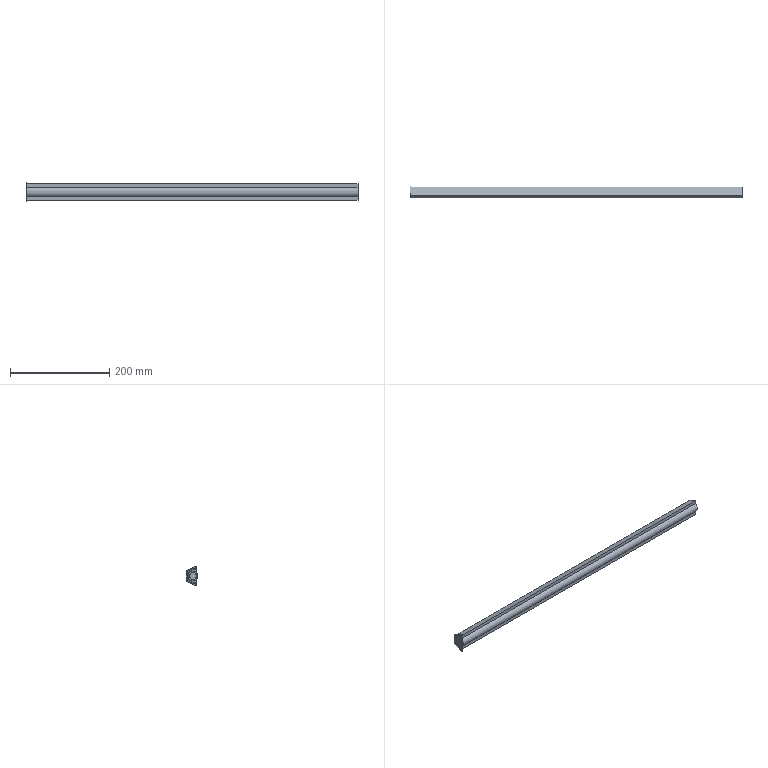Part | SolidWorks | features BaseBody 2, ICE 1 | 2 solids | 25 faces | box 670 x 24 x 40.186 mm | volume 190097 mm3 | plane 21 | cylinder 4 | commonest cylinder face diameters 14 x2 20 x2
STEP:
#1=CARTESIAN_POINT('',(-503.717,-23.698,18.335));
#2=VERTEX_POINT('',#1);
#3=CARTESIAN_POINT('',(-1171.717,-23.698,18.335));
#4=VERTEX_POINT('',#3);
#5=CARTESIAN_POINT('',(-6.717,-23.698,18.335));
#6=DIRECTION('',(-1.,0.,0.));
#7=VECTOR('',#6,1000.);
#8=LINE('',#5,#7);
#9=EDGE_CURVE('',#2,#4,#8,.T.);
#10=ORIENTED_EDGE('',*,*,#9,.F.);
#11=CARTESIAN_POINT('',(-503.717,-25.698,18.335));
#12=VERTEX_POINT('',#11);
#13=CARTESIAN_POINT('',(-503.717,-23.698,18.335));
#14=DIRECTION('',(0.,-1.,0.));
#15=VECTOR('',#14,1000.);
#16=LINE('',#13,#15);
#17=EDGE_CURVE('',#2,#12,#16,.T.);
#18=ORIENTED_EDGE('',*,*,#17,.T.);
#19=CARTESIAN_POINT('',(-1171.717,-25.698,18.335));
#20=VERTEX_POINT('',#19);
#21=CARTESIAN_POINT('',(-1171.717,-25.698,18.335));
#22=DIRECTION('',(1.,0.,0.));
#23=VECTOR('',#22,1000.);
#24=LINE('',#21,#23);
#25=EDGE_CURVE('',#20,#12,#24,.T.);
#26=ORIENTED_EDGE('',*,*,#25,.F.);
#27=CARTESIAN_POINT('',(-1171.717,-23.698,18.335));
#28=DIRECTION('',(0.,-1.,0.));
#29=VECTOR('',#28,1000.);
#30=LINE('',#27,#29);
#31=EDGE_CURVE('',#4,#20,#30,.T.);
#32=ORIENTED_EDGE('',*,*,#31,.F.);
#33=EDGE_LOOP('',(#10,#18,#26,#32));
#34=FACE_OUTER_BOUND('',#33,.T.);
#35=CARTESIAN_POINT('',(-6.717,-23.698,18.335));
#36=DIRECTION('',(0.,0.,-1.));
#37=DIRECTION('',(-1.,0.,0.));
#38=AXIS2_PLACEMENT_3D('',#35,#36,#37);
#39=PLANE('',#38);
#40=ADVANCED_FACE('',(#34),#39,.T.);
#41=CARTESIAN_POINT('',(-503.717,-8.698,17.685));
#42=VERTEX_POINT('',#41);
#43=CARTESIAN_POINT('',(-1171.717,-8.698,17.685));
#44=VERTEX_POINT('',#43);
#45=CARTESIAN_POINT('',(-6.717,-8.698,17.685));
#46=DIRECTION('',(-1.,0.,0.));
#47=VECTOR('',#46,1000.);
#48=LINE('',#45,#47);
#49=EDGE_CURVE('',#42,#44,#48,.T.);
#50=ORIENTED_EDGE('',*,*,#49,.F.);
#51=CARTESIAN_POINT('',(-503.717,-8.698,-1.015));
#52=VERTEX_POINT('',#51);
#53=CARTESIAN_POINT('',(-503.717,-8.698,17.685));
#54=DIRECTION('',(0.,0.,-1.));
#55=VECTOR('',#54,1000.);
#56=LINE('',#53,#55);
#57=EDGE_CURVE('',#42,#52,#56,.T.);
#58=ORIENTED_EDGE('',*,*,#57,.T.);
#59=CARTESIAN_POINT('',(-1171.717,-8.698,-1.015));
#60=VERTEX_POINT('',#59);
#61=CARTESIAN_POINT('',(-1171.717,-8.698,-1.015));
#62=DIRECTION('',(1.,0.,0.));
#63=VECTOR('',#62,1000.);
#64=LINE('',#61,#63);
#65=EDGE_CURVE('',#60,#52,#64,.T.);
#66=ORIENTED_EDGE('',*,*,#65,.F.);
#67=CARTESIAN_POINT('',(-1171.717,-8.698,17.685));
#68=DIRECTION('',(0.,0.,-1.));
#69=VECTOR('',#68,1000.);
#70=LINE('',#67,#69);
#71=EDGE_CURVE('',#44,#60,#70,.T.);
#72=ORIENTED_EDGE('',*,*,#71,.F.);
#73=EDGE_LOOP('',(#50,#58,#66,#72));
#74=FACE_OUTER_BOUND('',#73,.T.);
#75=CARTESIAN_POINT('',(-6.717,-8.698,17.685));
#76=DIRECTION('',(0.,1.,0.));
#77=DIRECTION('',(0.,0.,-1.));
#78=AXIS2_PLACEMENT_3D('',#75,#76,#77);
#79=PLANE('',#78);
#80=ADVANCED_FACE('',(#74),#79,.T.);
#81=ORIENTED_EDGE('',*,*,#65,.T.);
#82=CARTESIAN_POINT('',(-503.717,-25.698,-8.665));
#83=VERTEX_POINT('',#82);
#84=CARTESIAN_POINT('',(-503.717,-8.698,-1.015));
#85=DIRECTION('',(0.,-0.9119,-0.4104));
#86=VECTOR('',#85,1000.);
#87=LINE('',#84,#86);
#88=EDGE_CURVE('',#52,#83,#87,.T.);
#89=ORIENTED_EDGE('',*,*,#88,.T.);
#90=CARTESIAN_POINT('',(-1171.717,-25.698,-8.665));
#91=VERTEX_POINT('',#90);
#92=CARTESIAN_POINT('',(-1171.717,-25.698,-8.665));
#93=DIRECTION('',(1.,0.,0.));
#94=VECTOR('',#93,1000.);
#95=LINE('',#92,#94);
#96=EDGE_CURVE('',#91,#83,#95,.T.);
#97=ORIENTED_EDGE('',*,*,#96,.F.);
#98=CARTESIAN_POINT('',(-1171.717,-8.698,-1.015));
#99=DIRECTION('',(0.,-0.9119,-0.4104));
#100=VECTOR('',#99,1000.);
#101=LINE('',#98,#100);
#102=EDGE_CURVE('',#60,#91,#101,.T.);
#103=ORIENTED_EDGE('',*,*,#102,.F.);
#104=EDGE_LOOP('',(#81,#89,#97,#103));
#105=FACE_OUTER_BOUND('',#104,.T.);
#106=CARTESIAN_POINT('',(-6.717,-8.698,-1.015));
#107=DIRECTION('',(0.,0.4104,-0.9119));
#108=DIRECTION('',(-1.,0.,0.));
#109=AXIS2_PLACEMENT_3D('',#106,#107,#108);
#110=PLANE('',#109);
#111=ADVANCED_FACE('',(#105),#110,.T.);
#112=CARTESIAN_POINT('',(-503.717,-25.698,-1.665));
#113=VERTEX_POINT('',#112);
#114=CARTESIAN_POINT('',(-1171.717,-25.698,-1.665));
#115=VERTEX_POINT('',#114);
#116=CARTESIAN_POINT('',(-6.717,-25.698,-1.665));
#117=DIRECTION('',(-1.,0.,0.));
#118=VECTOR('',#117,1000.);
#119=LINE('',#116,#118);
#120=EDGE_CURVE('',#113,#115,#119,.T.);
#121=ORIENTED_EDGE('',*,*,#120,.F.);
#122=CARTESIAN_POINT('',(-503.717,-23.698,-1.665));
#123=VERTEX_POINT('',#122);
#124=CARTESIAN_POINT('',(-503.717,-25.698,-1.665));
#125=DIRECTION('',(0.,1.,0.));
#126=VECTOR('',#125,1000.);
#127=LINE('',#124,#126);
#128=EDGE_CURVE('',#113,#123,#127,.T.);
#129=ORIENTED_EDGE('',*,*,#128,.T.);
#130=CARTESIAN_POINT('',(-1171.717,-23.698,-1.665));
#131=VERTEX_POINT('',#130);
#132=CARTESIAN_POINT('',(-1171.717,-23.698,-1.665));
#133=DIRECTION('',(1.,0.,0.));
#134=VECTOR('',#133,1000.);
#135=LINE('',#132,#134);
#136=EDGE_CURVE('',#131,#123,#135,.T.);
#137=ORIENTED_EDGE('',*,*,#136,.F.);
#138=CARTESIAN_POINT('',(-1171.717,-25.698,-1.665));
#139=DIRECTION('',(0.,1.,0.));
#140=VECTOR('',#139,1000.);
#141=LINE('',#138,#140);
#142=EDGE_CURVE('',#115,#131,#141,.T.);
#143=ORIENTED_EDGE('',*,*,#142,.F.);
#144=EDGE_LOOP('',(#121,#129,#137,#143));
#145=FACE_OUTER_BOUND('',#144,.T.);
#146=CARTESIAN_POINT('',(-6.717,-25.698,-1.665));
#147=DIRECTION('',(0.,0.,1.));
#148=DIRECTION('',(0.,-1.,0.));
#149=AXIS2_PLACEMENT_3D('',#146,#147,#148);
#150=PLANE('',#149);
#151=ADVANCED_FACE('',(#145),#150,.T.);
#152=ORIENTED_EDGE('',*,*,#136,.T.);
#153=CARTESIAN_POINT('',(-503.717,-23.698,-5.572));
#154=VERTEX_POINT('',#153);
#155=CARTESIAN_POINT('',(-503.717,-23.698,-1.665));
#156=DIRECTION('',(0.,0.,-1.));
#157=VECTOR('',#156,1000.);
#158=LINE('',#155,#157);
#159=EDGE_CURVE('',#123,#154,#158,.T.);
#160=ORIENTED_EDGE('',*,*,#159,.T.);
#161=CARTESIAN_POINT('',(-1171.717,-23.698,-5.572));
#162=VERTEX_POINT('',#161);
#163=CARTESIAN_POINT('',(-1171.717,-23.698,-5.572));
#164=DIRECTION('',(1.,0.,0.));
#165=VECTOR('',#164,1000.);
#166=LINE('',#163,#165);
#167=EDGE_CURVE('',#162,#154,#166,.T.);
#168=ORIENTED_EDGE('',*,*,#167,.F.);
#169=CARTESIAN_POINT('',(-1171.717,-23.698,-1.665));
#170=DIRECTION('',(0.,0.,-1.));
#171=VECTOR('',#170,1000.);
#172=LINE('',#169,#171);
#173=EDGE_CURVE('',#131,#162,#172,.T.);
#174=ORIENTED_EDGE('',*,*,#173,.F.);
#175=EDGE_LOOP('',(#152,#160,#168,#174));
#176=FACE_OUTER_BOUND('',#175,.T.);
#177=CARTESIAN_POINT('',(-6.717,-23.698,-1.665));
#178=DIRECTION('',(0.,1.,0.));
#179=DIRECTION('',(0.,0.,-1.));
#180=AXIS2_PLACEMENT_3D('',#177,#178,#179);
#181=PLANE('',#180);
#182=ADVANCED_FACE('',(#176),#181,.T.);
#183=ORIENTED_EDGE('',*,*,#167,.T.);
#184=CARTESIAN_POINT('',(-503.717,-10.698,0.2778));
#185=VERTEX_POINT('',#184);
#186=CARTESIAN_POINT('',(-503.717,-23.698,-5.572));
#187=DIRECTION('',(0.,0.9119,0.4104));
#188=VECTOR('',#187,1000.);
#189=LINE('',#186,#188);
#190=EDGE_CURVE('',#154,#185,#189,.T.);
#191=ORIENTED_EDGE('',*,*,#190,.T.);
#192=CARTESIAN_POINT('',(-1171.717,-10.698,0.2778));
#193=VERTEX_POINT('',#192);
#194=CARTESIAN_POINT('',(-1171.717,-10.698,0.2778));
#195=DIRECTION('',(1.,0.,0.));
#196=VECTOR('',#195,1000.);
#197=LINE('',#194,#196);
#198=EDGE_CURVE('',#193,#185,#197,.T.);
#199=ORIENTED_EDGE('',*,*,#198,.F.);
#200=CARTESIAN_POINT('',(-1171.717,-23.698,-5.572));
#201=DIRECTION('',(0.,0.9119,0.4104));
#202=VECTOR('',#201,1000.);
#203=LINE('',#200,#202);
#204=EDGE_CURVE('',#162,#193,#203,.T.);
#205=ORIENTED_EDGE('',*,*,#204,.F.);
#206=EDGE_LOOP('',(#183,#191,#199,#205));
#207=FACE_OUTER_BOUND('',#206,.T.);
#208=CARTESIAN_POINT('',(-6.717,-23.698,-5.572));
#209=DIRECTION('',(0.,-0.4104,0.9119));
#210=DIRECTION('',(-1.,0.,0.));
#211=AXIS2_PLACEMENT_3D('',#208,#209,#210);
#212=PLANE('',#211);
#213=ADVANCED_FACE('',(#207),#212,.T.);
#214=ORIENTED_EDGE('',*,*,#198,.T.);
#215=CARTESIAN_POINT('',(-503.717,-10.698,16.391));
#216=VERTEX_POINT('',#215);
#217=CARTESIAN_POINT('',(-503.717,-10.698,0.2778));
#218=DIRECTION('',(0.,0.,1.));
#219=VECTOR('',#218,1000.);
#220=LINE('',#217,#219);
#221=EDGE_CURVE('',#185,#216,#220,.T.);
#222=ORIENTED_EDGE('',*,*,#221,.T.);
#223=CARTESIAN_POINT('',(-1171.717,-10.698,16.391));
#224=VERTEX_POINT('',#223);
#225=CARTESIAN_POINT('',(-1171.717,-10.698,16.391));
#226=DIRECTION('',(1.,0.,0.));
#227=VECTOR('',#226,1000.);
#228=LINE('',#225,#227);
#229=EDGE_CURVE('',#224,#216,#228,.T.);
#230=ORIENTED_EDGE('',*,*,#229,.F.);
#231=CARTESIAN_POINT('',(-1171.717,-10.698,0.2778));
#232=DIRECTION('',(0.,0.,1.));
#233=VECTOR('',#232,1000.);
#234=LINE('',#231,#233);
#235=EDGE_CURVE('',#193,#224,#234,.T.);
#236=ORIENTED_EDGE('',*,*,#235,.F.);
#237=EDGE_LOOP('',(#214,#222,#230,#236));
#238=FACE_OUTER_BOUND('',#237,.T.);
#239=CARTESIAN_POINT('',(-6.717,-10.698,0.2778));
#240=DIRECTION('',(0.,-1.,0.));
#241=DIRECTION('',(0.,0.,-1.));
#242=AXIS2_PLACEMENT_3D('',#239,#240,#241);
#243=PLANE('',#242);
#244=ADVANCED_FACE('',(#238),#243,.T.);
#245=ORIENTED_EDGE('',*,*,#229,.T.);
#246=CARTESIAN_POINT('',(-503.717,-23.698,22.241));
#247=VERTEX_POINT('',#246);
#248=CARTESIAN_POINT('',(-503.717,-10.698,16.391));
#249=DIRECTION('',(0.,-0.9119,0.4104));
#250=VECTOR('',#249,1000.);
#251=LINE('',#248,#250);
#252=EDGE_CURVE('',#216,#247,#251,.T.);
#253=ORIENTED_EDGE('',*,*,#252,.T.);
#254=CARTESIAN_POINT('',(-1171.717,-23.698,22.241));
#255=VERTEX_POINT('',#254);
#256=CARTESIAN_POINT('',(-1171.717,-23.698,22.241));
#257=DIRECTION('',(1.,0.,0.));
#258=VECTOR('',#257,1000.);
#259=LINE('',#256,#258);
#260=EDGE_CURVE('',#255,#247,#259,.T.);
#261=ORIENTED_EDGE('',*,*,#260,.F.);
#262=CARTESIAN_POINT('',(-1171.717,-10.698,16.391));
#263=DIRECTION('',(0.,-0.9119,0.4104));
#264=VECTOR('',#263,1000.);
#265=LINE('',#262,#264);
#266=EDGE_CURVE('',#224,#255,#265,.T.);
#267=ORIENTED_EDGE('',*,*,#266,.F.);
#268=EDGE_LOOP('',(#245,#253,#261,#267));
#269=FACE_OUTER_BOUND('',#268,.T.);
#270=CARTESIAN_POINT('',(-6.717,-10.698,16.391));
#271=DIRECTION('',(0.,-0.4104,-0.9119));
#272=DIRECTION('',(0.,-0.9119,0.4104));
#273=AXIS2_PLACEMENT_3D('',#270,#271,#272);
#274=PLANE('',#273);
#275=ADVANCED_FACE('',(#269),#274,.T.);
#276=ORIENTED_EDGE('',*,*,#260,.T.);
#277=CARTESIAN_POINT('',(-503.717,-23.698,22.241));
#278=DIRECTION('',(0.,0.,-1.));
#279=VECTOR('',#278,1000.);
#280=LINE('',#277,#279);
#281=EDGE_CURVE('',#247,#2,#280,.T.);
#282=ORIENTED_EDGE('',*,*,#281,.T.);
#283=ORIENTED_EDGE('',*,*,#9,.T.);
#284=CARTESIAN_POINT('',(-1171.717,-23.698,22.241));
#285=DIRECTION('',(0.,0.,-1.));
#286=VECTOR('',#285,1000.);
#287=LINE('',#284,#286);
#288=EDGE_CURVE('',#255,#4,#287,.T.);
#289=ORIENTED_EDGE('',*,*,#288,.F.);
#290=EDGE_LOOP('',(#276,#282,#283,#289));
#291=FACE_OUTER_BOUND('',#290,.T.);
#292=CARTESIAN_POINT('',(-6.717,-23.698,22.241));
#293=DIRECTION('',(0.,1.,0.));
#294=DIRECTION('',(1.,0.,0.));
#295=AXIS2_PLACEMENT_3D('',#292,#293,#294);
#296=PLANE('',#295);
#297=ADVANCED_FACE('',(#291),#296,.T.);
#298=ORIENTED_EDGE('',*,*,#25,.T.);
#299=CARTESIAN_POINT('',(-503.717,-25.698,25.335));
#300=VERTEX_POINT('',#299);
#301=CARTESIAN_POINT('',(-503.717,-25.698,-8.665));
#302=DIRECTION('',(0.,0.,1.));
#303=VECTOR('',#302,1000.);
#304=LINE('',#301,#303);
#305=EDGE_CURVE('',#12,#300,#304,.T.);
#306=ORIENTED_EDGE('',*,*,#305,.T.);
#307=CARTESIAN_POINT('',(-1171.717,-25.698,25.335));
#308=VERTEX_POINT('',#307);
#309=CARTESIAN_POINT('',(-1171.717,-25.698,25.335));
#310=DIRECTION('',(1.,0.,0.));
#311=VECTOR('',#310,1000.);
#312=LINE('',#309,#311);
#313=EDGE_CURVE('',#308,#300,#312,.T.);
#314=ORIENTED_EDGE('',*,*,#313,.F.);
#315=CARTESIAN_POINT('',(-1171.717,-25.698,25.335));
#316=DIRECTION('',(0.,0.,-1.));
#317=VECTOR('',#316,1000.);
#318=LINE('',#315,#317);
#319=EDGE_CURVE('',#308,#20,#318,.T.);
#320=ORIENTED_EDGE('',*,*,#319,.T.);
#321=EDGE_LOOP('',(#298,#306,#314,#320));
#322=FACE_OUTER_BOUND('',#321,.T.);
#323=CARTESIAN_POINT('',(-6.717,-25.698,-8.665));
#324=DIRECTION('',(0.,-1.,0.));
#325=DIRECTION('',(0.,0.,-1.));
#326=AXIS2_PLACEMENT_3D('',#323,#324,#325);
#327=PLANE('',#326);
#328=ADVANCED_FACE('',(#322),#327,.T.);
#329=ORIENTED_EDGE('',*,*,#96,.T.);
#330=CARTESIAN_POINT('',(-503.717,-25.698,-8.665));
#331=DIRECTION('',(0.,0.,1.));
#332=VECTOR('',#331,1000.);
#333=LINE('',#330,#332);
#334=EDGE_CURVE('',#83,#113,#333,.T.);
#335=ORIENTED_EDGE('',*,*,#334,.T.);
#336=ORIENTED_EDGE('',*,*,#120,.T.);
#337=CARTESIAN_POINT('',(-1171.717,-25.698,-1.665));
#338=DIRECTION('',(0.,0.,-1.));
#339=VECTOR('',#338,1000.);
#340=LINE('',#337,#339);
#341=EDGE_CURVE('',#115,#91,#340,.T.);
#342=ORIENTED_EDGE('',*,*,#341,.T.);
#343=EDGE_LOOP('',(#329,#335,#336,#342));
#344=FACE_OUTER_BOUND('',#343,.T.);
#345=CARTESIAN_POINT('',(-6.717,-25.698,-8.665));
#346=DIRECTION('',(0.,-1.,0.));
#347=DIRECTION('',(0.,0.,-1.));
#348=AXIS2_PLACEMENT_3D('',#345,#346,#347);
#349=PLANE('',#348);
#350=ADVANCED_FACE('',(#344),#349,.T.);
#351=ORIENTED_EDGE('',*,*,#313,.T.);
#352=CARTESIAN_POINT('',(-503.717,-25.698,25.335));
#353=DIRECTION('',(0.,0.9119,-0.4104));
#354=VECTOR('',#353,1000.);
#355=LINE('',#352,#354);
#356=EDGE_CURVE('',#300,#42,#355,.T.);
#357=ORIENTED_EDGE('',*,*,#356,.T.);
#358=ORIENTED_EDGE('',*,*,#49,.T.);
#359=CARTESIAN_POINT('',(-1171.717,-8.698,17.685));
#360=DIRECTION('',(0.,-0.9119,0.4104));
#361=VECTOR('',#360,1000.);
#362=LINE('',#359,#361);
#363=EDGE_CURVE('',#44,#308,#362,.T.);
#364=ORIENTED_EDGE('',*,*,#363,.T.);
#365=EDGE_LOOP('',(#351,#357,#358,#364));
#366=FACE_OUTER_BOUND('',#365,.T.);
#367=CARTESIAN_POINT('',(-6.717,-25.698,25.335));
#368=DIRECTION('',(0.,0.4104,0.9119));
#369=DIRECTION('',(1.,0.,0.));
#370=AXIS2_PLACEMENT_3D('',#367,#368,#369);
#371=PLANE('',#370);
#372=ADVANCED_FACE('',(#366),#371,.T.);
#373=CARTESIAN_POINT('',(-1173.717,-6.698,18.978));
#374=VERTEX_POINT('',#373);
#375=CARTESIAN_POINT('',(-1173.717,-27.698,28.428));
#376=VERTEX_POINT('',#375);
#377=CARTESIAN_POINT('',(-1173.717,-6.698,18.978));
#378=DIRECTION('',(0.,-0.9119,0.4104));
#379=VECTOR('',#378,1000.);
#380=LINE('',#377,#379);
#381=EDGE_CURVE('',#374,#376,#380,.T.);
#382=ORIENTED_EDGE('',*,*,#381,.F.);
#383=CARTESIAN_POINT('',(-1173.717,-6.698,-2.309));
#384=VERTEX_POINT('',#383);
#385=CARTESIAN_POINT('',(-1173.717,-6.698,-2.309));
#386=DIRECTION('',(0.,0.,1.));
#387=VECTOR('',#386,1000.);
#388=LINE('',#385,#387);
#389=EDGE_CURVE('',#384,#374,#388,.T.);
#390=ORIENTED_EDGE('',*,*,#389,.F.);
#391=CARTESIAN_POINT('',(-1173.717,-27.698,-11.759));
#392=VERTEX_POINT('',#391);
#393=CARTESIAN_POINT('',(-1173.717,-27.698,-11.759));
#394=DIRECTION('',(0.,0.9119,0.4104));
#395=VECTOR('',#394,1000.);
#396=LINE('',#393,#395);
#397=EDGE_CURVE('',#392,#384,#396,.T.);
#398=ORIENTED_EDGE('',*,*,#397,.F.);
#399=CARTESIAN_POINT('',(-1173.717,-27.698,28.428));
#400=DIRECTION('',(0.,0.,-1.));
#401=VECTOR('',#400,1000.);
#402=LINE('',#399,#401);
#403=EDGE_CURVE('',#376,#392,#402,.T.);
#404=ORIENTED_EDGE('',*,*,#403,.F.);
#405=EDGE_LOOP('',(#382,#390,#398,#404));
#406=FACE_OUTER_BOUND('',#405,.T.);
#407=CARTESIAN_POINT('',(-1173.717,-17.198,8.335));
#408=DIRECTION('',(-1.,0.,0.));
#409=DIRECTION('',(0.,0.,1.));
#410=AXIS2_PLACEMENT_3D('',#407,#408,#409);
#411=PLANE('',#410);
#412=ADVANCED_FACE('',(#406),#411,.T.);
#413=ORIENTED_EDGE('',*,*,#142,.T.);
#414=ORIENTED_EDGE('',*,*,#173,.T.);
#415=ORIENTED_EDGE('',*,*,#204,.T.);
#416=ORIENTED_EDGE('',*,*,#235,.T.);
#417=ORIENTED_EDGE('',*,*,#266,.T.);
#418=ORIENTED_EDGE('',*,*,#288,.T.);
#419=ORIENTED_EDGE('',*,*,#31,.T.);
#420=ORIENTED_EDGE('',*,*,#319,.F.);
#421=ORIENTED_EDGE('',*,*,#363,.F.);
#422=ORIENTED_EDGE('',*,*,#71,.T.);
#423=ORIENTED_EDGE('',*,*,#102,.T.);
#424=ORIENTED_EDGE('',*,*,#341,.F.);
#425=EDGE_LOOP('',(#413,#414,#415,#416,#417,#418,#419,#420,#421,#422,#423,#424));
#426=FACE_BOUND('',#425,.T.);
#427=CARTESIAN_POINT('',(-1171.717,-27.698,28.428));
#428=VERTEX_POINT('',#427);
#429=CARTESIAN_POINT('',(-1171.717,-6.698,18.978));
#430=VERTEX_POINT('',#429);
#431=CARTESIAN_POINT('',(-1171.717,-27.698,28.428));
#432=DIRECTION('',(0.,0.9119,-0.4104));
#433=VECTOR('',#432,1000.);
#434=LINE('',#431,#433);
#435=EDGE_CURVE('',#428,#430,#434,.T.);
#436=ORIENTED_EDGE('',*,*,#435,.F.);
#437=CARTESIAN_POINT('',(-1171.717,-27.698,-11.759));
#438=VERTEX_POINT('',#437);
#439=CARTESIAN_POINT('',(-1171.717,-27.698,-11.759));
#440=DIRECTION('',(0.,0.,1.));
#441=VECTOR('',#440,1000.);
#442=LINE('',#439,#441);
#443=EDGE_CURVE('',#438,#428,#442,.T.);
#444=ORIENTED_EDGE('',*,*,#443,.F.);
#445=CARTESIAN_POINT('',(-1171.717,-6.698,-2.309));
#446=VERTEX_POINT('',#445);
#447=CARTESIAN_POINT('',(-1171.717,-6.698,-2.309));
#448=DIRECTION('',(0.,-0.9119,-0.4104));
#449=VECTOR('',#448,1000.);
#450=LINE('',#447,#449);
#451=EDGE_CURVE('',#446,#438,#450,.T.);
#452=ORIENTED_EDGE('',*,*,#451,.F.);
#453=CARTESIAN_POINT('',(-1171.717,-6.698,18.978));
#454=DIRECTION('',(0.,0.,-1.));
#455=VECTOR('',#454,1000.);
#456=LINE('',#453,#455);
#457=EDGE_CURVE('',#430,#446,#456,.T.);
#458=ORIENTED_EDGE('',*,*,#457,.F.);
#459=EDGE_LOOP('',(#436,#444,#452,#458));
#460=FACE_OUTER_BOUND('',#459,.T.);
#461=CARTESIAN_POINT('',(-1171.717,-17.198,8.335));
#462=DIRECTION('',(1.,0.,0.));
#463=DIRECTION('',(0.,1.,0.));
#464=AXIS2_PLACEMENT_3D('',#461,#462,#463);
#465=PLANE('',#464);
#466=ADVANCED_FACE('',(#426,#460),#465,.T.);
#467=ORIENTED_EDGE('',*,*,#381,.T.);
#468=CARTESIAN_POINT('',(-1171.717,-27.698,28.428));
#469=DIRECTION('',(-1.,0.,0.));
#470=VECTOR('',#469,1000.);
#471=LINE('',#468,#470);
#472=EDGE_CURVE('',#428,#376,#471,.T.);
#473=ORIENTED_EDGE('',*,*,#472,.F.);
#474=ORIENTED_EDGE('',*,*,#435,.T.);
#475=CARTESIAN_POINT('',(-1173.717,-6.698,18.978));
#476=DIRECTION('',(1.,0.,0.));
#477=VECTOR('',#476,1000.);
#478=LINE('',#475,#477);
#479=EDGE_CURVE('',#374,#430,#478,.T.);
#480=ORIENTED_EDGE('',*,*,#479,.F.);
#481=EDGE_LOOP('',(#467,#473,#474,#480));
#482=FACE_OUTER_BOUND('',#481,.T.);
#483=CARTESIAN_POINT('',(-1173.717,-6.698,18.978));
#484=DIRECTION('',(0.,0.4104,0.9119));
#485=DIRECTION('',(1.,0.,0.));
#486=AXIS2_PLACEMENT_3D('',#483,#484,#485);
#487=PLANE('',#486);
#488=ADVANCED_FACE('',(#482),#487,.T.);
#489=ORIENTED_EDGE('',*,*,#403,.T.);
#490=CARTESIAN_POINT('',(-1171.717,-27.698,-11.759));
#491=DIRECTION('',(-1.,0.,0.));
#492=VECTOR('',#491,1000.);
#493=LINE('',#490,#492);
#494=EDGE_CURVE('',#438,#392,#493,.T.);
#495=ORIENTED_EDGE('',*,*,#494,.F.);
#496=ORIENTED_EDGE('',*,*,#443,.T.);
#497=ORIENTED_EDGE('',*,*,#472,.T.);
#498=EDGE_LOOP('',(#489,#495,#496,#497));
#499=FACE_OUTER_BOUND('',#498,.T.);
#500=CARTESIAN_POINT('',(-1173.717,-27.698,28.428));
#501=DIRECTION('',(0.,-1.,0.));
#502=DIRECTION('',(0.,0.,-1.));
#503=AXIS2_PLACEMENT_3D('',#500,#501,#502);
#504=PLANE('',#503);
#505=ADVANCED_FACE('',(#499),#504,.T.);
#506=ORIENTED_EDGE('',*,*,#397,.T.);
#507=CARTESIAN_POINT('',(-1171.717,-6.698,-2.309));
#508=DIRECTION('',(-1.,0.,0.));
#509=VECTOR('',#508,1000.);
#510=LINE('',#507,#509);
#511=EDGE_CURVE('',#446,#384,#510,.T.);
#512=ORIENTED_EDGE('',*,*,#511,.F.);
#513=ORIENTED_EDGE('',*,*,#451,.T.);
#514=ORIENTED_EDGE('',*,*,#494,.T.);
#515=EDGE_LOOP('',(#506,#512,#513,#514));
#516=FACE_OUTER_BOUND('',#515,.T.);
#517=CARTESIAN_POINT('',(-1173.717,-27.698,-11.759));
#518=DIRECTION('',(0.,0.4104,-0.9119));
#519=DIRECTION('',(-1.,0.,0.));
#520=AXIS2_PLACEMENT_3D('',#517,#518,#519);
#521=PLANE('',#520);
#522=ADVANCED_FACE('',(#516),#521,.T.);
#523=ORIENTED_EDGE('',*,*,#389,.T.);
#524=ORIENTED_EDGE('',*,*,#479,.T.);
#525=ORIENTED_EDGE('',*,*,#457,.T.);
#526=ORIENTED_EDGE('',*,*,#511,.T.);
#527=EDGE_LOOP('',(#523,#524,#525,#526));
#528=FACE_OUTER_BOUND('',#527,.T.);
#529=CARTESIAN_POINT('',(-1173.717,-6.698,-2.309));
#530=DIRECTION('',(0.,1.,0.));
#531=DIRECTION('',(0.,0.,-1.));
#532=AXIS2_PLACEMENT_3D('',#529,#530,#531);
#533=PLANE('',#532);
#534=ADVANCED_FACE('',(#528),#533,.T.);
#535=ORIENTED_EDGE('',*,*,#88,.F.);
#536=ORIENTED_EDGE('',*,*,#57,.F.);
#537=ORIENTED_EDGE('',*,*,#356,.F.);
#538=ORIENTED_EDGE('',*,*,#305,.F.);
#539=ORIENTED_EDGE('',*,*,#17,.F.);
#540=ORIENTED_EDGE('',*,*,#281,.F.);
#541=ORIENTED_EDGE('',*,*,#252,.F.);
#542=ORIENTED_EDGE('',*,*,#221,.F.);
#543=ORIENTED_EDGE('',*,*,#190,.F.);
#544=ORIENTED_EDGE('',*,*,#159,.F.);
#545=ORIENTED_EDGE('',*,*,#128,.F.);
#546=ORIENTED_EDGE('',*,*,#334,.F.);
#547=EDGE_LOOP('',(#535,#536,#537,#538,#539,#540,#541,#542,#543,#544,#545,#546));
#548=FACE_OUTER_BOUND('',#547,.T.);
#549=CARTESIAN_POINT('',(-503.717,0.,0.));
#550=DIRECTION('',(1.,0.,0.));
#551=DIRECTION('',(0.,0.,-1.));
#552=AXIS2_PLACEMENT_3D('',#549,#550,#551);
#553=PLANE('',#552);
#554=ADVANCED_FACE('',(#548),#553,.T.);
#555=CLOSED_SHELL('',(#40,#80,#111,#151,#182,#213,#244,#275,#297,#328,#350,#372,#412,#466,#488,#505,#522,#534,#554));
#556=MANIFOLD_SOLID_BREP('',#555);
#557=CARTESIAN_POINT('',(-503.717,-20.698,18.335));
#558=VERTEX_POINT('',#557);
#559=CARTESIAN_POINT('',(-1171.717,-20.698,18.335));
#560=VERTEX_POINT('',#559);
#561=CARTESIAN_POINT('',(-6.717,-20.698,18.335));
#562=DIRECTION('',(-1.,0.,0.));
#563=VECTOR('',#562,1000.);
#564=LINE('',#561,#563);
#565=EDGE_CURVE('',#558,#560,#564,.T.);
#566=ORIENTED_EDGE('',*,*,#565,.F.);
#567=CARTESIAN_POINT('',(-503.717,-20.698,-1.665));
#568=VERTEX_POINT('',#567);
#569=CARTESIAN_POINT('',(-503.717,-20.698,8.335));
#570=DIRECTION('',(-1.,0.,0.));
#571=DIRECTION('',(0.,0.,-1.));
#572=AXIS2_PLACEMENT_3D('',#569,#570,#571);
#573=CIRCLE('',#572,10.);
#574=EDGE_CURVE('',#558,#568,#573,.T.);
#575=ORIENTED_EDGE('',*,*,#574,.T.);
#576=CARTESIAN_POINT('',(-1171.717,-20.698,-1.665));
#577=VERTEX_POINT('',#576);
#578=CARTESIAN_POINT('',(-1171.717,-20.698,-1.665));
#579=DIRECTION('',(1.,0.,0.));
#580=VECTOR('',#579,1000.);
#581=LINE('',#578,#580);
#582=EDGE_CURVE('',#577,#568,#581,.T.);
#583=ORIENTED_EDGE('',*,*,#582,.F.);
#584=CARTESIAN_POINT('',(-1171.717,-20.698,8.335));
#585=DIRECTION('',(1.,0.,0.));
#586=DIRECTION('',(0.,0.,-1.));
#587=AXIS2_PLACEMENT_3D('',#584,#585,#586);
#588=CIRCLE('',#587,10.);
#589=EDGE_CURVE('',#577,#560,#588,.T.);
#590=ORIENTED_EDGE('',*,*,#589,.T.);
#591=EDGE_LOOP('',(#566,#575,#583,#590));
#592=FACE_OUTER_BOUND('',#591,.T.);
#593=CARTESIAN_POINT('',(-1171.717,-20.698,8.335));
#594=DIRECTION('',(1.,0.,0.));
#595=DIRECTION('',(0.,0.,-1.));
#596=AXIS2_PLACEMENT_3D('',#593,#594,#595);
#597=CYLINDRICAL_SURFACE('',#596,10.);
#598=ADVANCED_FACE('',(#592),#597,.T.);
#599=ORIENTED_EDGE('',*,*,#582,.T.);
#600=CARTESIAN_POINT('',(-503.717,-20.698,8.335));
#601=DIRECTION('',(-1.,0.,0.));
#602=DIRECTION('',(0.,0.,-1.));
#603=AXIS2_PLACEMENT_3D('',#600,#601,#602);
#604=CIRCLE('',#603,10.);
#605=EDGE_CURVE('',#568,#558,#604,.T.);
#606=ORIENTED_EDGE('',*,*,#605,.T.);
#607=ORIENTED_EDGE('',*,*,#565,.T.);
#608=CARTESIAN_POINT('',(-1171.717,-20.698,8.335));
#609=DIRECTION('',(1.,0.,0.));
#610=DIRECTION('',(0.,0.,1.));
#611=AXIS2_PLACEMENT_3D('',#608,#609,#610);
#612=CIRCLE('',#611,10.);
#613=EDGE_CURVE('',#560,#577,#612,.T.);
#614=ORIENTED_EDGE('',*,*,#613,.T.);
#615=EDGE_LOOP('',(#599,#606,#607,#614));
#616=FACE_OUTER_BOUND('',#615,.T.);
#617=CARTESIAN_POINT('',(-1171.717,-20.698,8.335));
#618=DIRECTION('',(1.,0.,0.));
#619=DIRECTION('',(0.,0.,-1.));
#620=AXIS2_PLACEMENT_3D('',#617,#618,#619);
#621=CYLINDRICAL_SURFACE('',#620,10.);
#622=ADVANCED_FACE('',(#616),#621,.T.);
#623=CARTESIAN_POINT('',(-503.717,-20.698,1.335));
#624=VERTEX_POINT('',#623);
#625=CARTESIAN_POINT('',(-503.717,-20.698,15.335));
#626=VERTEX_POINT('',#625);
#627=CARTESIAN_POINT('',(-503.717,-20.698,8.335));
#628=DIRECTION('',(-1.,0.,0.));
#629=DIRECTION('',(0.,0.,-1.));
#630=AXIS2_PLACEMENT_3D('',#627,#628,#629);
#631=CIRCLE('',#630,7.);
#632=EDGE_CURVE('',#624,#626,#631,.T.);
#633=ORIENTED_EDGE('',*,*,#632,.F.);
#634=CARTESIAN_POINT('',(-1171.717,-20.698,1.335));
#635=VERTEX_POINT('',#634);
#636=CARTESIAN_POINT('',(-1171.717,-20.698,1.335));
#637=DIRECTION('',(1.,0.,0.));
#638=VECTOR('',#637,1000.);
#639=LINE('',#636,#638);
#640=EDGE_CURVE('',#635,#624,#639,.T.);
#641=ORIENTED_EDGE('',*,*,#640,.F.);
#642=CARTESIAN_POINT('',(-1171.717,-20.698,15.335));
#643=VERTEX_POINT('',#642);
#644=CARTESIAN_POINT('',(-1171.717,-20.698,8.335));
#645=DIRECTION('',(-1.,0.,0.));
#646=DIRECTION('',(0.,0.,-1.));
#647=AXIS2_PLACEMENT_3D('',#644,#645,#646);
#648=CIRCLE('',#647,7.);
#649=EDGE_CURVE('',#635,#643,#648,.T.);
#650=ORIENTED_EDGE('',*,*,#649,.T.);
#651=CARTESIAN_POINT('',(-6.717,-20.698,15.335));
#652=DIRECTION('',(-1.,0.,0.));
#653=VECTOR('',#652,1000.);
#654=LINE('',#651,#653);
#655=EDGE_CURVE('',#626,#643,#654,.T.);
#656=ORIENTED_EDGE('',*,*,#655,.F.);
#657=EDGE_LOOP('',(#633,#641,#650,#656));
#658=FACE_OUTER_BOUND('',#657,.T.);
#659=CARTESIAN_POINT('',(-1171.717,-20.698,8.335));
#660=DIRECTION('',(1.,0.,0.));
#661=DIRECTION('',(0.,0.,-1.));
#662=AXIS2_PLACEMENT_3D('',#659,#660,#661);
#663=CYLINDRICAL_SURFACE('',#662,7.);
#664=ADVANCED_FACE('',(#658),#663,.F.);
#665=CARTESIAN_POINT('',(-503.717,-20.698,8.335));
#666=DIRECTION('',(-1.,0.,0.));
#667=DIRECTION('',(0.,0.,-1.));
#668=AXIS2_PLACEMENT_3D('',#665,#666,#667);
#669=CIRCLE('',#668,7.);
#670=EDGE_CURVE('',#626,#624,#669,.T.);
#671=ORIENTED_EDGE('',*,*,#670,.F.);
#672=ORIENTED_EDGE('',*,*,#655,.T.);
#673=CARTESIAN_POINT('',(-1171.717,-20.698,8.335));
#674=DIRECTION('',(-1.,0.,0.));
#675=DIRECTION('',(0.,0.,1.));
#676=AXIS2_PLACEMENT_3D('',#673,#674,#675);
#677=CIRCLE('',#676,7.);
#678=EDGE_CURVE('',#643,#635,#677,.T.);
#679=ORIENTED_EDGE('',*,*,#678,.T.);
#680=ORIENTED_EDGE('',*,*,#640,.T.);
#681=EDGE_LOOP('',(#671,#672,#679,#680));
#682=FACE_OUTER_BOUND('',#681,.T.);
#683=CARTESIAN_POINT('',(-1171.717,-20.698,8.335));
#684=DIRECTION('',(1.,0.,0.));
#685=DIRECTION('',(0.,0.,-1.));
#686=AXIS2_PLACEMENT_3D('',#683,#684,#685);
#687=CYLINDRICAL_SURFACE('',#686,7.);
#688=ADVANCED_FACE('',(#682),#687,.F.);
#689=ORIENTED_EDGE('',*,*,#649,.F.);
#690=ORIENTED_EDGE('',*,*,#678,.F.);
#691=EDGE_LOOP('',(#689,#690));
#692=FACE_BOUND('',#691,.T.);
#693=ORIENTED_EDGE('',*,*,#589,.F.);
#694=ORIENTED_EDGE('',*,*,#613,.F.);
#695=EDGE_LOOP('',(#693,#694));
#696=FACE_OUTER_BOUND('',#695,.T.);
#697=CARTESIAN_POINT('',(-1171.717,-20.698,8.335));
#698=DIRECTION('',(-1.,0.,0.));
#699=DIRECTION('',(0.,0.,1.));
#700=AXIS2_PLACEMENT_3D('',#697,#698,#699);
#701=PLANE('',#700);
#702=ADVANCED_FACE('',(#692,#696),#701,.T.);
#703=ORIENTED_EDGE('',*,*,#605,.F.);
#704=ORIENTED_EDGE('',*,*,#574,.F.);
#705=EDGE_LOOP('',(#703,#704));
#706=FACE_OUTER_BOUND('',#705,.T.);
#707=ORIENTED_EDGE('',*,*,#632,.T.);
#708=ORIENTED_EDGE('',*,*,#670,.T.);
#709=EDGE_LOOP('',(#707,#708));
#710=FACE_BOUND('',#709,.T.);
#711=CARTESIAN_POINT('',(-503.717,0.,0.));
#712=DIRECTION('',(1.,0.,0.));
#713=DIRECTION('',(0.,0.,-1.));
#714=AXIS2_PLACEMENT_3D('',#711,#712,#713);
#715=PLANE('',#714);
#716=ADVANCED_FACE('',(#706,#710),#715,.T.);
#717=CLOSED_SHELL('',(#598,#622,#664,#688,#702,#716));
#718=MANIFOLD_SOLID_BREP('',#717);
#719=CARTESIAN_POINT('',(0.,0.,0.));
#720=DIRECTION('',(0.,0.,1.));
#721=DIRECTION('',(1.,0.,0.));
#722=AXIS2_PLACEMENT_3D('',#719,#720,#721);
#723=(LENGTH_UNIT()NAMED_UNIT(*)SI_UNIT(.MILLI.,.METRE.));
#724=UNCERTAINTY_MEASURE_WITH_UNIT(LENGTH_MEASURE(0.00001),#723,'','');
#725=(NAMED_UNIT(*)PLANE_ANGLE_UNIT()SI_UNIT($,.RADIAN.));
#726=(NAMED_UNIT(*)SI_UNIT($,.STERADIAN.)SOLID_ANGLE_UNIT());
#727=(GEOMETRIC_REPRESENTATION_CONTEXT(3)GLOBAL_UNCERTAINTY_ASSIGNED_CONTEXT((#724))GLOBAL_UNIT_ASSIGNED_CONTEXT((#723,#725,#726))REPRESENTATION_CONTEXT('',''));
#728=ADVANCED_BREP_SHAPE_REPRESENTATION('',(#556,#718,#722),#727);